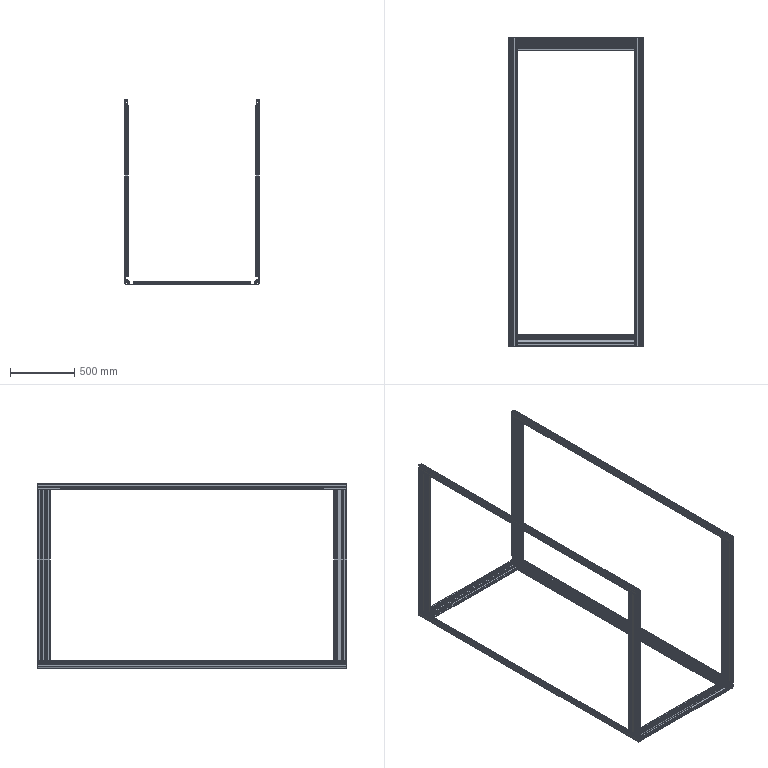Part | SolidWorks | features WeldMemberFeat 5, ICE 4, 3DProfileFeature 1, WeldmentFeature 1 | 13 solids | 1108 faces | box 1050 x 2416 x 1445 mm | volume 13308461 mm3 | plane 770 | cylinder 338 | commonest cylinder face diameters 0.6 x80 0.4 x65 15 x48 2 x24 0.24 x18 9 x18